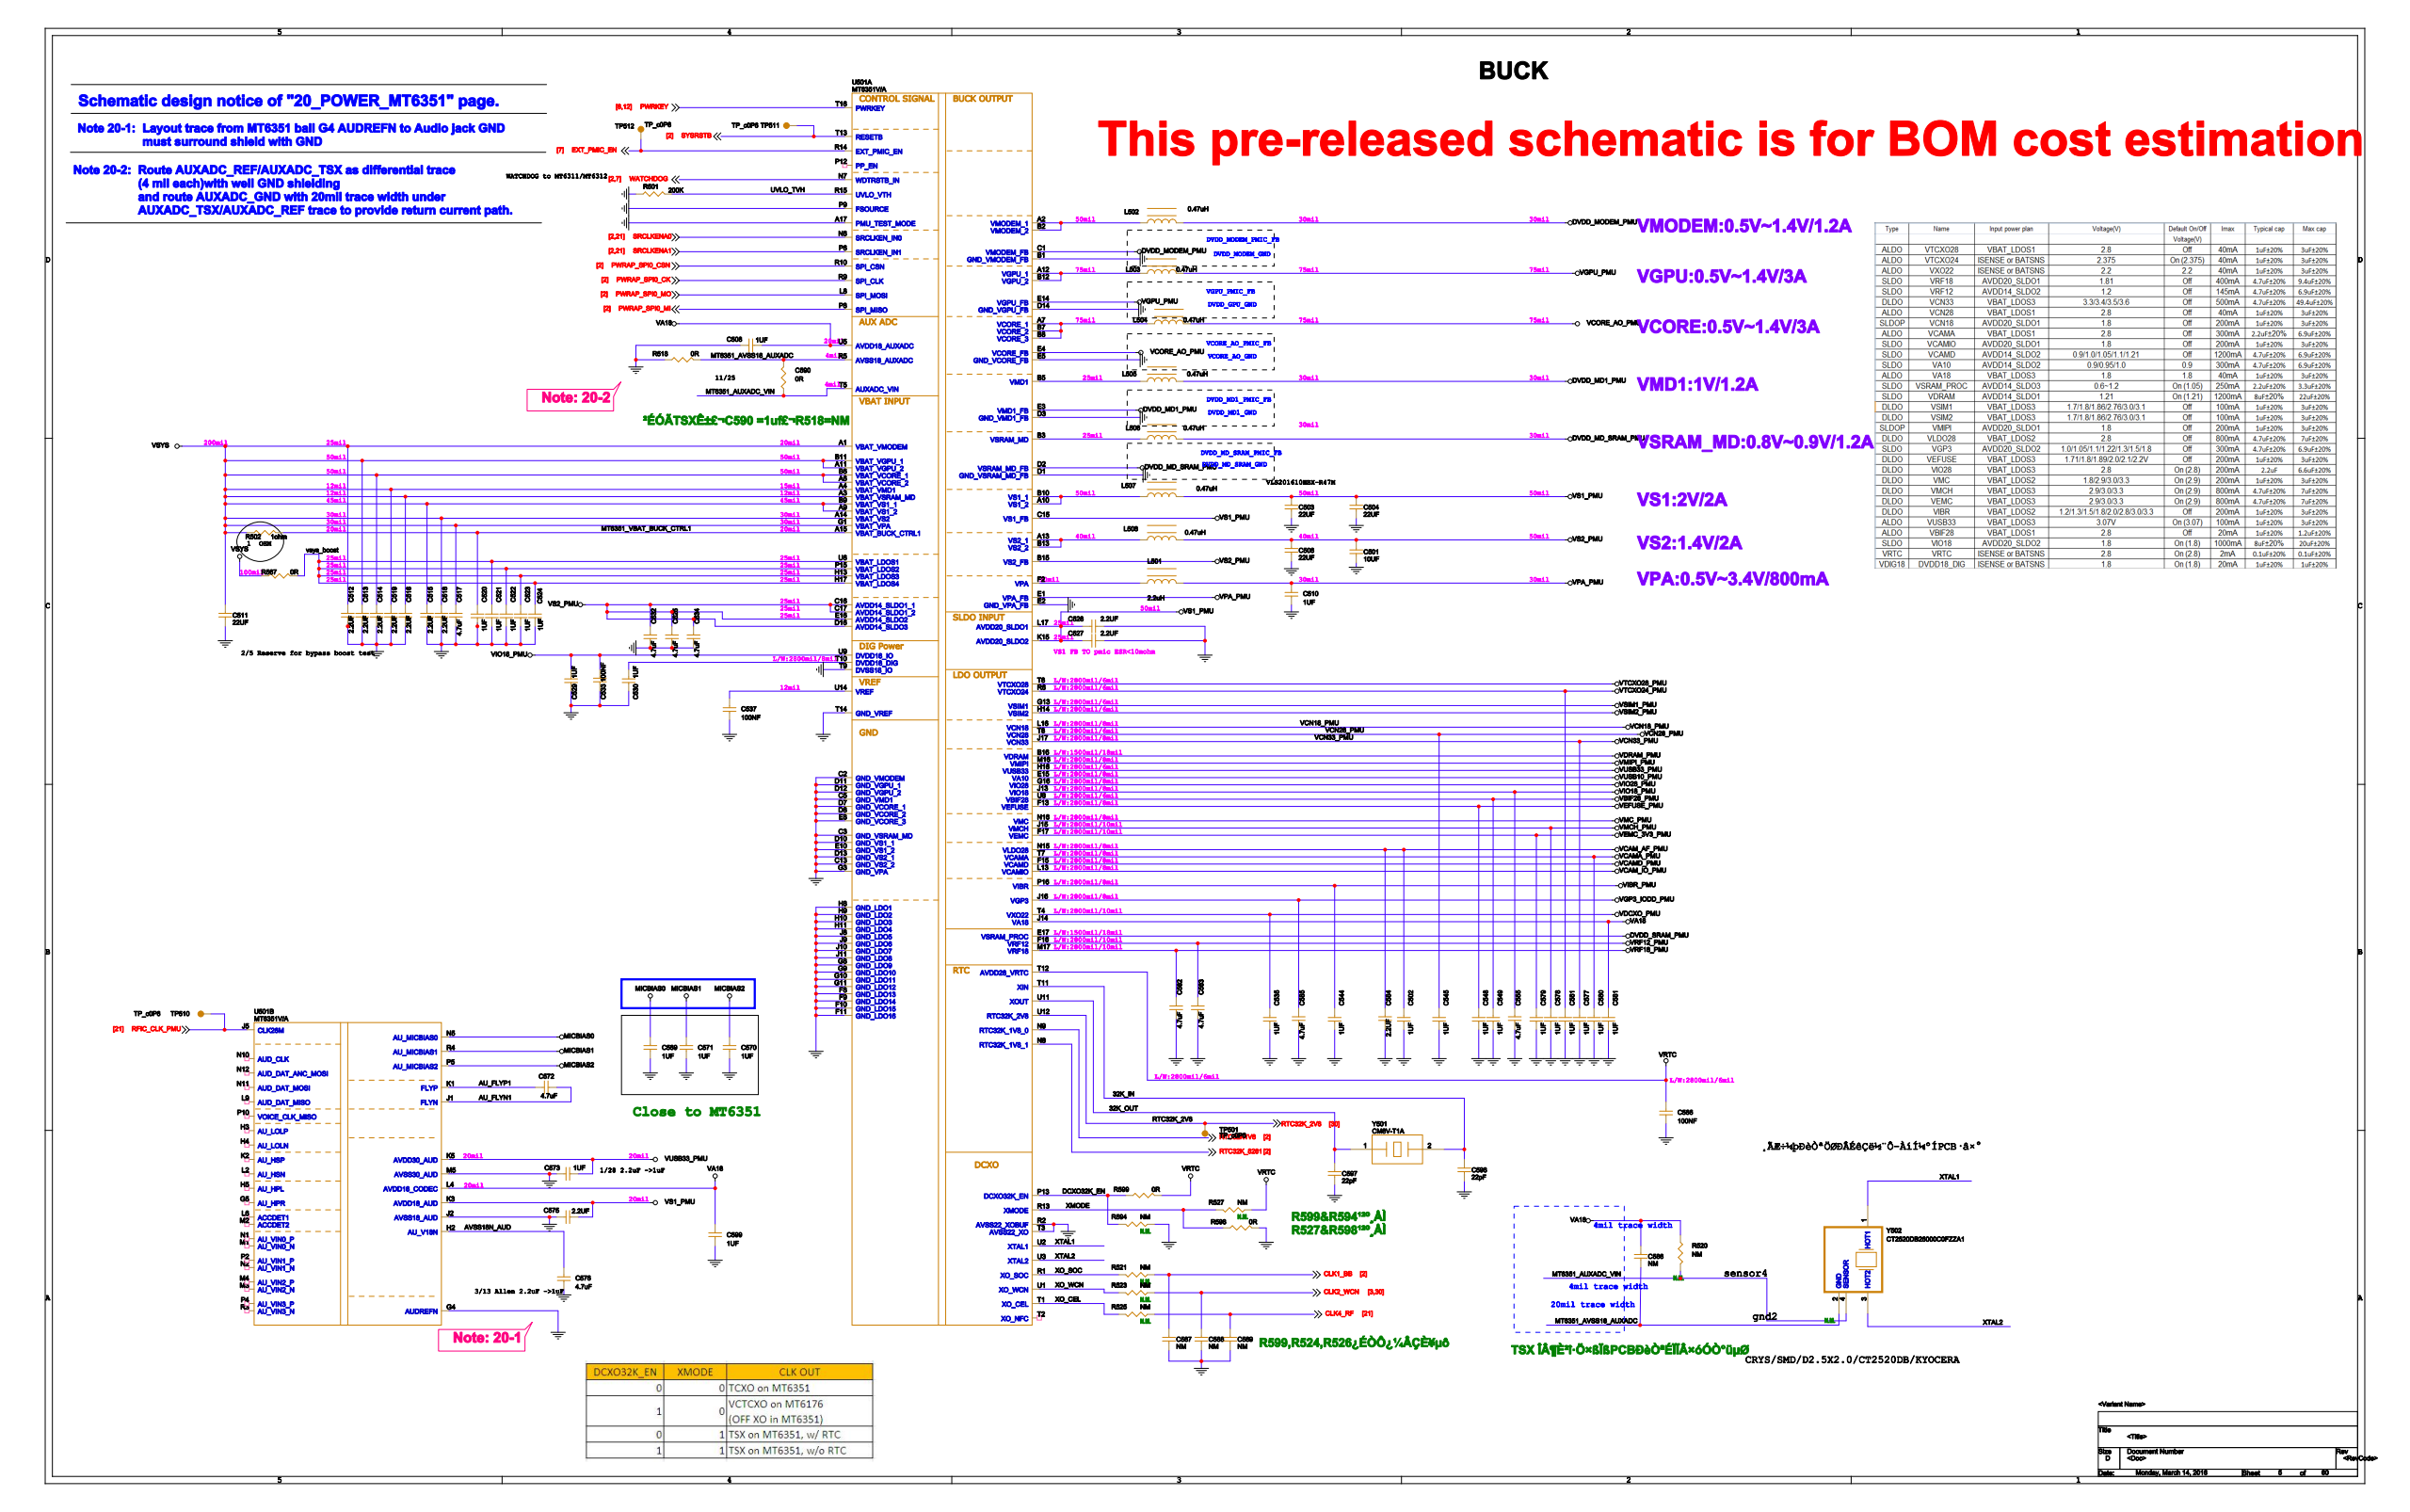Circuit board | Cadence Allegro | 1088 parts | 793 nets | one sheet of the schematic
Parts on this sheet (reference | value | footprint):
C501 | 10UF | 0402-BIG
C502 | 1UF | C0201
C503 | 22UF | 0603-BIG
C504 | 22UF | 0603-BIG
C506 | 22UF | 0603-BIG
C508 | 1UF | C0201
C510 | 1UF | C0201
C511 | 22UF | 0603-BIG
C512 | 2.2UF | 0402-BIG
C513 | 2.2UF | 0402-BIG
C514 | 2.2UF | 0402-BIG
C515 | 2.2UF | 0402-BIG
C516 | 2.2UF | 0402-BIG
C517
C518 | 2.2UF | 0402-BIG
C519 | 2.2UF | 0402-BIG
C520 | 1UF | C0201
C521 | 1UF | C0201
C522 | 1UF | C0201
C523 | 1UF | C0201
C524 | 1UF | C0201
C525 | 4.7uF | 0402-BIG
C527 | 2.2UF | 0402-BIG
C528 | 2.2UF | 0402-BIG
C529 | 1UF | C0201
C530 | 1UF | C0201
C532 | 4.7uF | 0402-BIG
C533 | 100NF | C0201
C534 | 4.7uF | 0402-BIG
C535 | 1UF | C0201
C537 | 100NF | C0201
C544 | 1UF | C0201
C545 | 1UF | C0201
C548 | 1UF | C0201
C549 | 1UF | C0201
C555 | 4.7uF | 0402-BIG
C561 | 1UF | C0201
C566 | 100NF | C0201
C569 | 1UF | C0201
C570 | 1UF | C0201
C571 | 1UF | C0201
C572 | 4.7uF | 0402-BIG
C573 | 1UF | C0201
C575 | 2.2UF | 0402-BIG
C576 | 4.7uF | 0402-BIG
C577 | 1UF | C0201
C578 | 1UF | C0201
C579 | 1UF | C0201
C580 | 1UF | C0201
C581 | 1UF | C0201
C582 | 4.7uF | 0402-BIG
C583 | 4.7uF | 0402-BIG
C584 | 2.2UF | 0402-BIG
C585 | 4.7uF | 0402-BIG
C586 | NM | 0201_NM
C587 | NM | 0201_NM
C588 | NM | 0201_NM
C589 | NM | 0201_NM
C590 | 0R | R0201
C597 | 22PF | C0201
C598 | 22PF | C0201
C599 | 1UF | C0201
L501 | 2.2uH | L2520_MPIA252010E
L502 | 0.47uH | L2016_VLS201610HBX-1
L503 | 0.47uH | L2016_MAKK2016
L504 | 0.47uH | L2016_MAKK2016
L505 | 0.47uH | L2016_VLS201610HBX-1
L506 | 0.47uH | L2016_VLS201610HBX-1
L507 | 0.47uH | L2016_MPIA201610-R47M-LF
L508 | 0.47uH | L2016_MPIA201610-R47M-LF
R501 | 200K | R0201
R502 | 1ohm | R0201
R518 | 0R | R0201
R520
R521
R523
R525
R527
R567 | 0R | R0603
R594
R598 | 0R | R0201
R599 | 0R | R0201
TP501 | TP_c0P6 | TP_C0P6
TP510 | TP_c0P6 | TP_C0P6
TP511 | TP_c0P6 | TP_C0P6
TP512 | TP_c0P6 | TP_C0P6
U501 | MT6351V/A | MT6351
Y501 | CM8V-T1A | Y2_CM8V-T1A
Y502
Nets of these parts (net: part-pin ...):
GND: C501-2 C502-1 C503-2 C504-2 C506-2 C508-1 C510-1 C511-2 C512-2 C513-2 C514-2 C515-2 C516-2 C517-2 C518-2 C519-2 C520-1 C521-1 C522-1 C523-1 C524-1 C525-2 C527-1 C528-1 C529-1 C530-1 C532-2 C533-2 C534-2 C535-1 C537-1 C544-1 C545-1 C548-1 C549-1 C555-2 C561-1 C566-1 C569-2 C570-2 C571-2 C573-2 C575-2 C576-1 C577-1 C578-1 C579-1 C580-1 C581-1 C582-2 C583-2 C584-2 C585-2 C587-2 C588-2 C589-2 C597-2 C598-2 C599-2 R501-1 R518-1 R594-1 R598-2 U501-A17 U501-B1 U501-C2 U501-C3 U501-C5 U501-C13 U501-D1 U501-D3 U501-D7 U501-D8 U501-D10 U501-D11 U501-D12 U501-D13 U501-D14 U501-E2 U501-E5 U501-E8 U501-E10 U501-F8 U501-F9 U501-F10 U501-F11 U501-G3 U501-G4 U501-G8 U501-G9 U501-G10 U501-G11 U501-H8 U501-H9 U501-H10 U501-H11 U501-J2 U501-J8 U501-J9 U501-J10 U501-J11 U501-M5 U501-P9 U501-R2 U501-T3 U501-T9 U501-T14
VMIPI_PMU: U501-M16
VSYS: C511-1 C512-1 C513-1 C514-1 C515-1 C516-1 C517-1 C518-1 C519-1 R502-1 R567-1 U501-A1 U501-A3 U501-A4 U501-A6 U501-A9 U501-A11 U501-A14 U501-B6 U501-B9 U501-B11 U501-G1
MT6351_VBAT_BUCK_CTRL1: C520-2 R502-2 U501-A15
VIO28_PMU: U501-G16
VDRAM_PMU: U501-B16
PWRAP_SPI0_CK: U501-R9
PWRAP_SPI0_CSN: U501-R10
PWRAP_SPI0_MI: U501-P8
PWRAP_SPI0_MO: U501-L8
RTC32K1V8: U501-N9
SRCLKENA0: U501-N6
SRCLKENA1: U501-P6
SYSRSTB: TP511-1 U501-T13
WATCHDOG: U501-N7
DVDD_MD1_PMU: L505-2 U501-E3
VGPU_PMU: L503-2 U501-E14
DVDD_MODEM_PMU: L502-2 U501-C1
DVDD_SRAM_PMU: U501-E17
DVDD_MD_SRAM_PMU: L506-2 U501-D2
VCORE_AO_PMU: L504-2 U501-E4
VUSB10_PMU: U501-E15
VIO18_PMU: C529-2 C533-1 C555-1 U501-J13 U501-U9
VTCXO28_PMU: U501-T6
VUSB33_PMU: C573-1 U501-H16 U501-K5
VMC_PMU: U501-N16
VSIM1_PMU: U501-G13
VSIM2_PMU: U501-H14
VEFUSE_PMU: C548-2 U501-F13
EXT_PMIC_EN: TP512-1 U501-R14
32K_OUT: C597-1 Y501-1 U501-U11
32K_IN: C598-1 Y501-2 U501-T11
RTC32K_8281: U501-N8
MT6351_AVSS18_AUXADC: C586-2 C590-2 R518-2 Y502-2 U501-R5
XTAL1: Y502-1 U501-U2
XTAL2: Y502-3 U501-U3
MT6351_AUXADC_VIN: C590-1 R520-2 Y502-4 U501-T5
VRTC: C566-2 R527-1 R599-2 U501-T12
RTC32K_2V8: TP501-1 U501-U12
N3240103: L502-1 U501-A2 U501-B2
N16418208: L505-1 U501-B5
N3253323: L506-1 U501-B3
VMCH_PMU: C578-2 U501-J15
VCAM_AF_PMU: C502-2 C584-1 U501-N15
VPA_PMU: C510-2 L501-2 U501-E1
VIBR_PMU: C544-2 U501-P16
VA18: C508-2 C581-2 C586-1 C599-1 R520-1 U501-J14 U501-L4 U501-U5
VSYS_BOOST: C521-2 C522-2 C523-2 C524-2 R567-2 U501-H13 U501-H17 U501-P15 U501-U6
N3301654: C530-2 U501-T10
VDCXO_PMU: C535-2 U501-T4
VCN28_PMU: C545-2 U501-T8
VBIF28_PMU: C549-2 U501-U8
VTCXO24_PMU: C561-2 U501-R6
MICBIAS0: C569-1 U501-N5
MICBIAS2: C570-1 U501-P5
MICBIAS1: C571-1 U501-R4
VCN33_PMU: C577-2 U501-J17
VEMC_3V3_PMU: C579-2 U501-F17
VCAMA_PMU: C580-2 U501-T7
VCAM_IO_PMU: U501-L13
VS1_PMU: C503-1 C504-1 C527-2 C528-2 C575-1 L507-2 U501-C15 U501-K3 U501-K15 U501-L17
AU_FLYN1: C572-1 U501-J1
AU_FLYP1: C572-2 U501-K1
VS2_PMU: C501-1 C506-1 C525-1 C532-1 C534-1 L508-2 U501-B15 U501-C16 U501-C17 U501-D16 U501-E16
AVSS18N_AUD: C576-2 U501-H2
VRF18_PMU: C582-1 U501-M17
VRF12_PMU: C583-1 U501-F16
VGP3_IODD_PMU: C585-1 U501-J16
PWRKEY: U501-T16
N16509706: C537-2 U501-U14
CLK1_BB: C587-1 R521-1
CLK2_WCN: C588-1 R523-1
CLK4_RF: C589-1 R525-1
N3254294: L501-1 U501-F2
N16416444: L503-1 U501-A12 U501-B12
N16417438: L504-1 U501-A7 U501-B7 U501-B8
N16413760: L507-1 U501-A10 U501-B10
N16413721: L508-1 U501-A13 U501-B13
XO_SOC: R521-2 U501-R1
XO_WCN: R523-2 U501-U1
XO_CEL: R525-2 U501-T1
XMODE: R527-2 R598-1 U501-R13
DCXO32K_EN: R594-2 R599-1 U501-P13
UVLO_TVH: R501-2 U501-R15
RFIC_CLK_PMU: TP510-1 U501-J5
VCAMD_PMU: U501-F15
VCN18_PMU: U501-L16